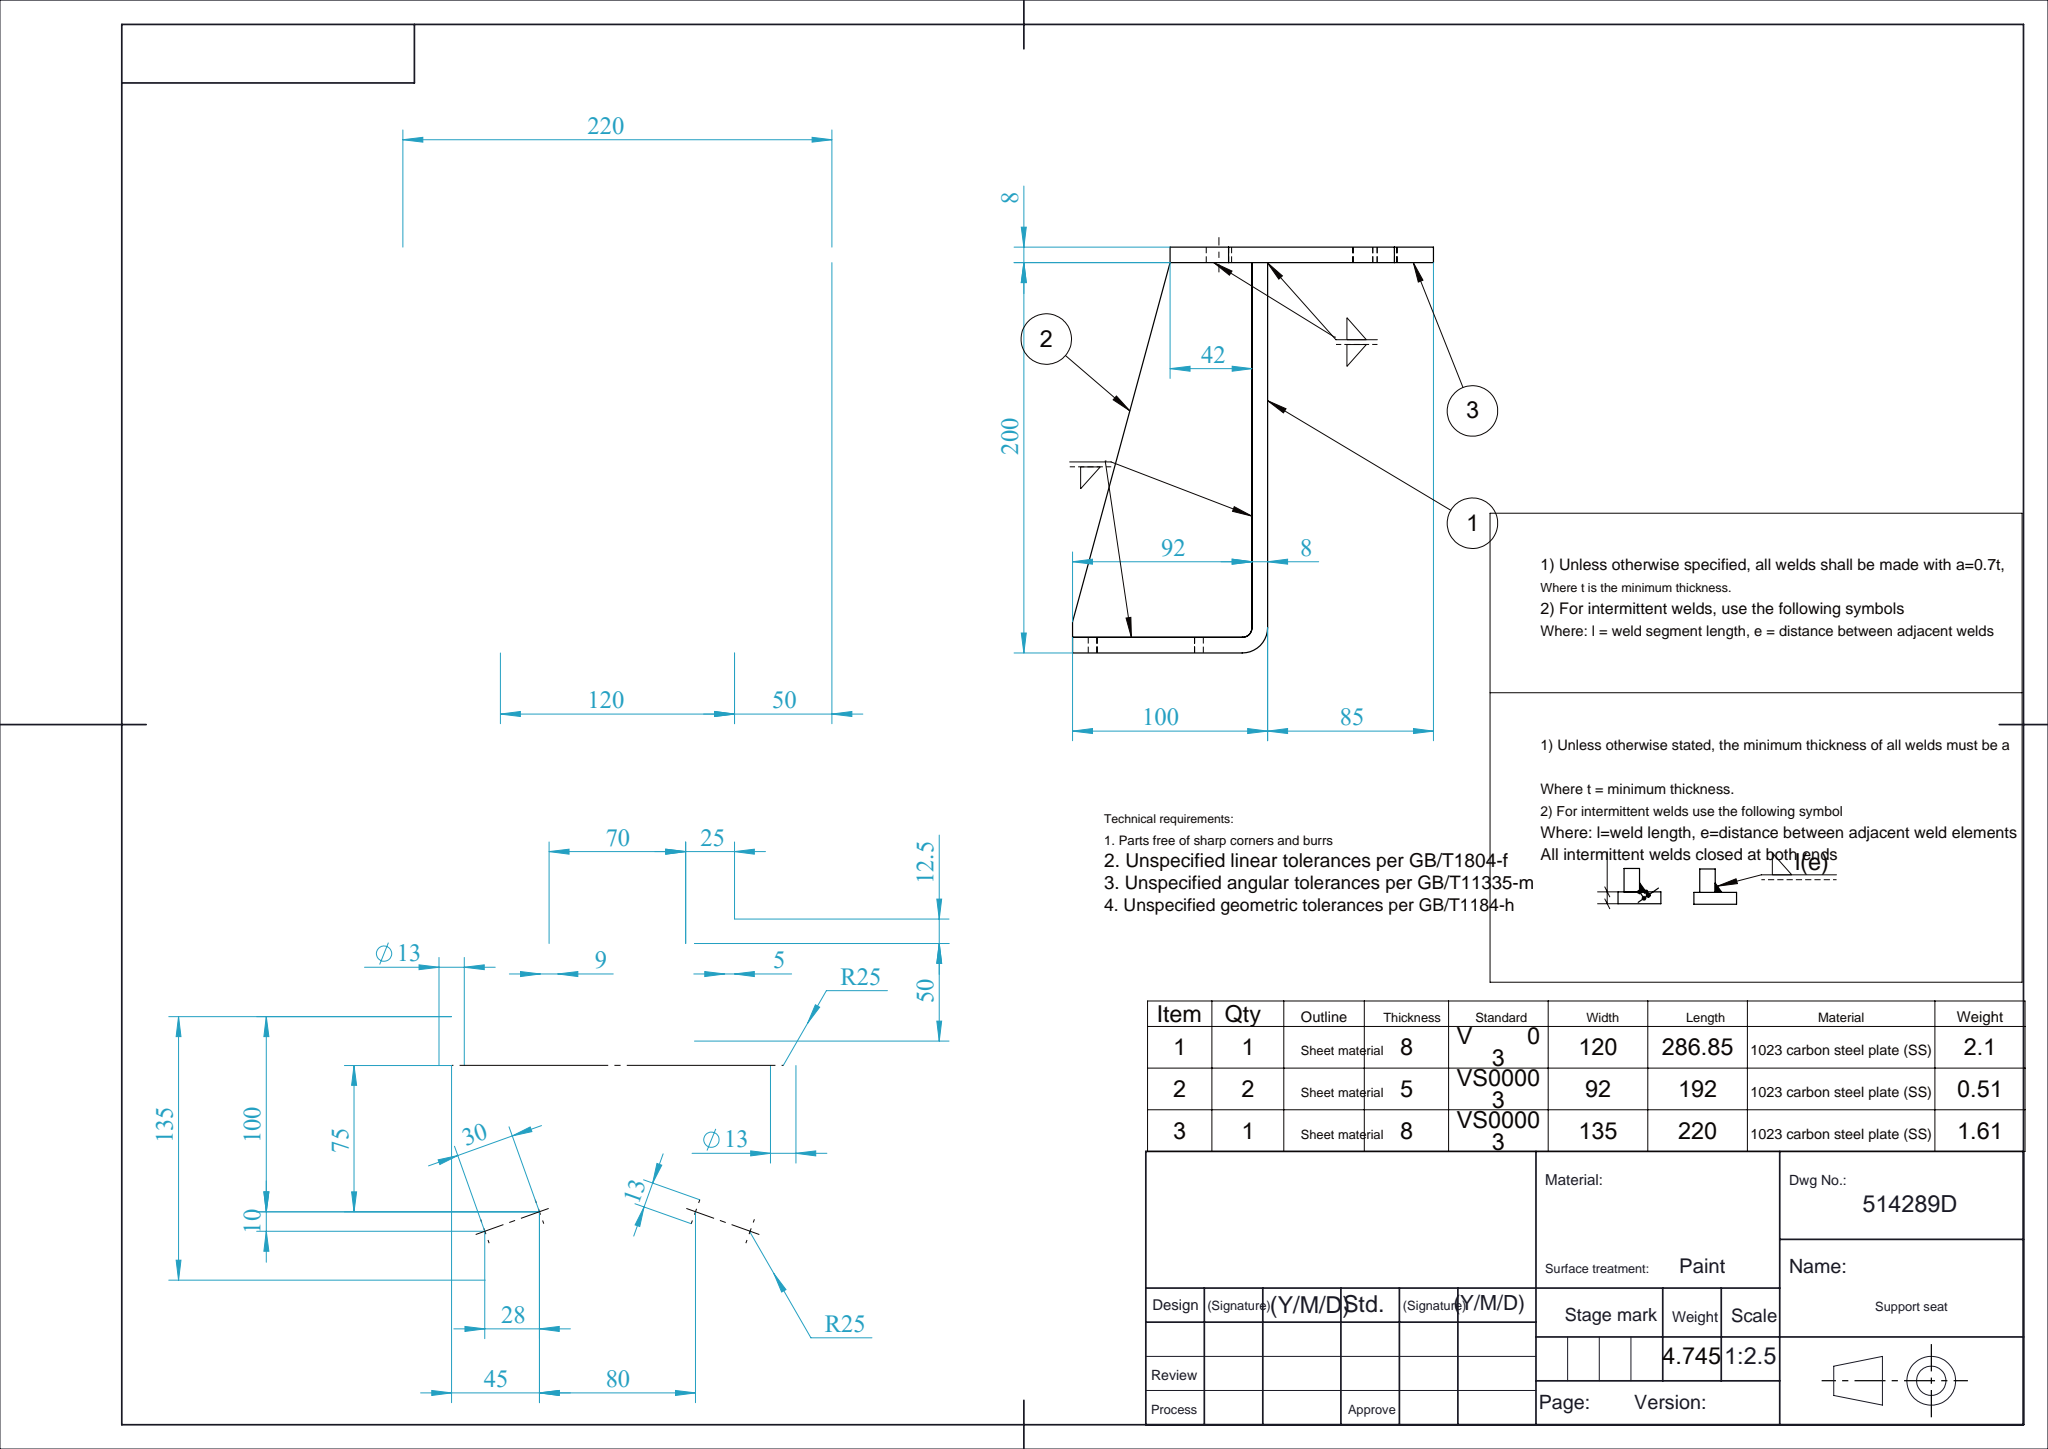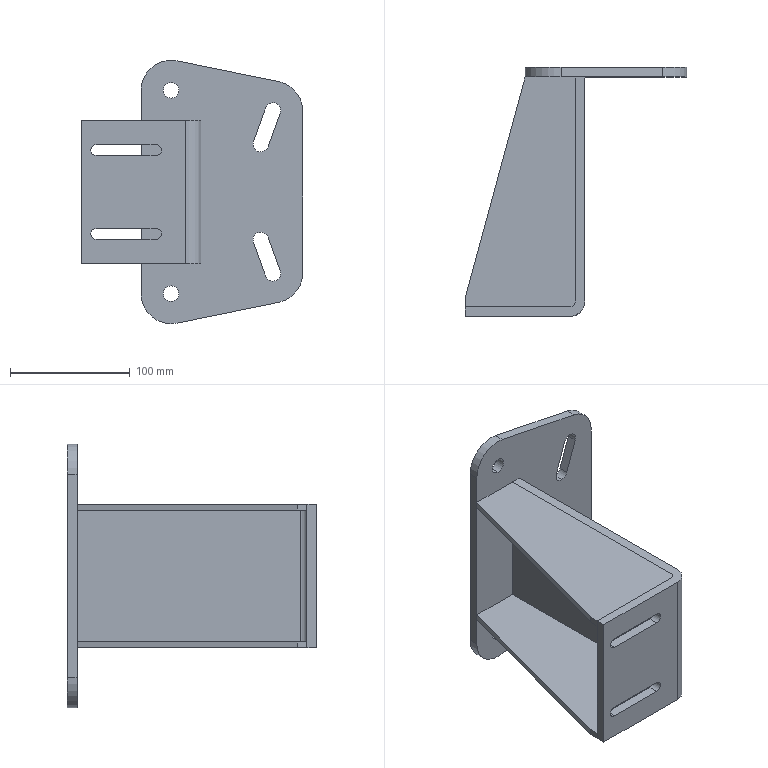Part | SolidWorks | 4 solids | 59 faces | box 185 x 208 x 220 mm | volume 603876 mm3 | plane 36 | cylinder 23 | commonest cylinder face diameters 13 x10 50 x5 9 x4 10 x3 26 x1